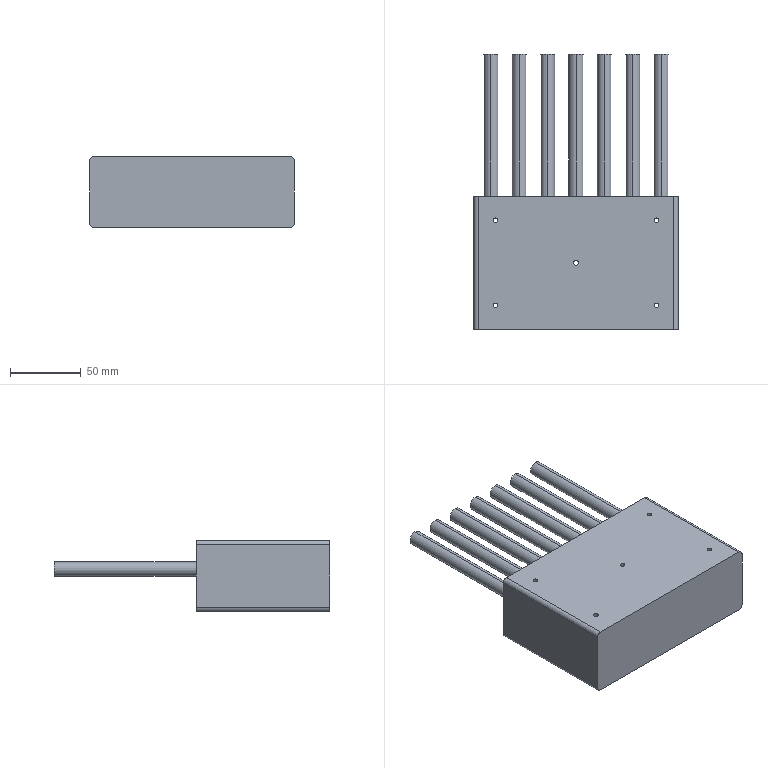Part | SolidWorks | features Extrusion 1, Fillet 1, HoleWzd 1, ICE 1 | 8 solids | 48 faces | box 144 x 194 x 50 mm | volume 728913 mm3 | cylinder 28 | plane 20 | commonest cylinder face diameters 10 x14 3.3 x10 6 x4
STEP:
#1=CARTESIAN_POINT('',(0.,147.,35.));
#2=VERTEX_POINT('',#1);
#3=CARTESIAN_POINT('',(0.,147.,25.));
#4=VERTEX_POINT('',#3);
#5=CARTESIAN_POINT('',(0.,147.,30.));
#6=DIRECTION('',(0.,1.,0.));
#7=DIRECTION('',(0.,0.,1.));
#8=AXIS2_PLACEMENT_3D('',#5,#6,#7);
#9=CIRCLE('',#8,5.);
#10=EDGE_CURVE('',#2,#4,#9,.T.);
#11=ORIENTED_EDGE('',*,*,#10,.F.);
#12=CARTESIAN_POINT('',(0.,47.,35.));
#13=VERTEX_POINT('',#12);
#14=CARTESIAN_POINT('',(0.,147.,35.));
#15=DIRECTION('',(0.,-1.,0.));
#16=VECTOR('',#15,1000.);
#17=LINE('',#14,#16);
#18=EDGE_CURVE('',#2,#13,#17,.T.);
#19=ORIENTED_EDGE('',*,*,#18,.T.);
#20=CARTESIAN_POINT('',(0.,47.,25.));
#21=VERTEX_POINT('',#20);
#22=CARTESIAN_POINT('',(0.,47.,30.));
#23=DIRECTION('',(0.,1.,0.));
#24=DIRECTION('',(0.,0.,1.));
#25=AXIS2_PLACEMENT_3D('',#22,#23,#24);
#26=CIRCLE('',#25,5.);
#27=EDGE_CURVE('',#13,#21,#26,.T.);
#28=ORIENTED_EDGE('',*,*,#27,.T.);
#29=CARTESIAN_POINT('',(0.,147.,25.));
#30=DIRECTION('',(0.,-1.,0.));
#31=VECTOR('',#30,1000.);
#32=LINE('',#29,#31);
#33=EDGE_CURVE('',#4,#21,#32,.T.);
#34=ORIENTED_EDGE('',*,*,#33,.F.);
#35=EDGE_LOOP('',(#11,#19,#28,#34));
#36=FACE_OUTER_BOUND('',#35,.T.);
#37=CARTESIAN_POINT('',(0.,147.,30.));
#38=DIRECTION('',(0.,-1.,0.));
#39=DIRECTION('',(0.,0.,-1.));
#40=AXIS2_PLACEMENT_3D('',#37,#38,#39);
#41=CYLINDRICAL_SURFACE('',#40,5.);
#42=ADVANCED_FACE('',(#36),#41,.T.);
#43=ORIENTED_EDGE('',*,*,#18,.F.);
#44=CARTESIAN_POINT('',(0.,147.,30.));
#45=DIRECTION('',(0.,1.,0.));
#46=DIRECTION('',(0.,0.,1.));
#47=AXIS2_PLACEMENT_3D('',#44,#45,#46);
#48=CIRCLE('',#47,5.);
#49=EDGE_CURVE('',#4,#2,#48,.T.);
#50=ORIENTED_EDGE('',*,*,#49,.F.);
#51=ORIENTED_EDGE('',*,*,#33,.T.);
#52=CARTESIAN_POINT('',(0.,47.,30.));
#53=DIRECTION('',(0.,1.,0.));
#54=DIRECTION('',(0.,0.,1.));
#55=AXIS2_PLACEMENT_3D('',#52,#53,#54);
#56=CIRCLE('',#55,5.);
#57=EDGE_CURVE('',#21,#13,#56,.T.);
#58=ORIENTED_EDGE('',*,*,#57,.T.);
#59=EDGE_LOOP('',(#43,#50,#51,#58));
#60=FACE_OUTER_BOUND('',#59,.T.);
#61=CARTESIAN_POINT('',(0.,147.,30.));
#62=DIRECTION('',(0.,-1.,0.));
#63=DIRECTION('',(0.,0.,-1.));
#64=AXIS2_PLACEMENT_3D('',#61,#62,#63);
#65=CYLINDRICAL_SURFACE('',#64,5.);
#66=ADVANCED_FACE('',(#60),#65,.T.);
#67=ORIENTED_EDGE('',*,*,#49,.T.);
#68=ORIENTED_EDGE('',*,*,#10,.T.);
#69=EDGE_LOOP('',(#67,#68));
#70=FACE_OUTER_BOUND('',#69,.T.);
#71=CARTESIAN_POINT('',(0.,147.,30.));
#72=DIRECTION('',(0.,1.,0.));
#73=DIRECTION('',(0.,0.,1.));
#74=AXIS2_PLACEMENT_3D('',#71,#72,#73);
#75=PLANE('',#74);
#76=ADVANCED_FACE('',(#70),#75,.T.);
#77=ORIENTED_EDGE('',*,*,#57,.F.);
#78=ORIENTED_EDGE('',*,*,#27,.F.);
#79=EDGE_LOOP('',(#77,#78));
#80=FACE_OUTER_BOUND('',#79,.T.);
#81=CARTESIAN_POINT('',(0.,47.,30.));
#82=DIRECTION('',(0.,1.,0.));
#83=DIRECTION('',(0.,0.,1.));
#84=AXIS2_PLACEMENT_3D('',#81,#82,#83);
#85=PLANE('',#84);
#86=ADVANCED_FACE('',(#80),#85,.F.);
#87=CLOSED_SHELL('',(#42,#66,#76,#86));
#88=MANIFOLD_SOLID_BREP('',#87);
#89=CARTESIAN_POINT('',(20.,147.,35.));
#90=VERTEX_POINT('',#89);
#91=CARTESIAN_POINT('',(20.,147.,25.));
#92=VERTEX_POINT('',#91);
#93=CARTESIAN_POINT('',(20.,147.,30.));
#94=DIRECTION('',(0.,1.,0.));
#95=DIRECTION('',(0.,0.,1.));
#96=AXIS2_PLACEMENT_3D('',#93,#94,#95);
#97=CIRCLE('',#96,5.);
#98=EDGE_CURVE('',#90,#92,#97,.T.);
#99=ORIENTED_EDGE('',*,*,#98,.F.);
#100=CARTESIAN_POINT('',(20.,47.,35.));
#101=VERTEX_POINT('',#100);
#102=CARTESIAN_POINT('',(20.,147.,35.));
#103=DIRECTION('',(0.,-1.,0.));
#104=VECTOR('',#103,1000.);
#105=LINE('',#102,#104);
#106=EDGE_CURVE('',#90,#101,#105,.T.);
#107=ORIENTED_EDGE('',*,*,#106,.T.);
#108=CARTESIAN_POINT('',(20.,47.,25.));
#109=VERTEX_POINT('',#108);
#110=CARTESIAN_POINT('',(20.,47.,30.));
#111=DIRECTION('',(0.,1.,0.));
#112=DIRECTION('',(0.,0.,1.));
#113=AXIS2_PLACEMENT_3D('',#110,#111,#112);
#114=CIRCLE('',#113,5.);
#115=EDGE_CURVE('',#101,#109,#114,.T.);
#116=ORIENTED_EDGE('',*,*,#115,.T.);
#117=CARTESIAN_POINT('',(20.,147.,25.));
#118=DIRECTION('',(0.,-1.,0.));
#119=VECTOR('',#118,1000.);
#120=LINE('',#117,#119);
#121=EDGE_CURVE('',#92,#109,#120,.T.);
#122=ORIENTED_EDGE('',*,*,#121,.F.);
#123=EDGE_LOOP('',(#99,#107,#116,#122));
#124=FACE_OUTER_BOUND('',#123,.T.);
#125=CARTESIAN_POINT('',(20.,147.,30.));
#126=DIRECTION('',(0.,-1.,0.));
#127=DIRECTION('',(0.,0.,-1.));
#128=AXIS2_PLACEMENT_3D('',#125,#126,#127);
#129=CYLINDRICAL_SURFACE('',#128,5.);
#130=ADVANCED_FACE('',(#124),#129,.T.);
#131=ORIENTED_EDGE('',*,*,#106,.F.);
#132=CARTESIAN_POINT('',(20.,147.,30.));
#133=DIRECTION('',(0.,1.,0.));
#134=DIRECTION('',(0.,0.,1.));
#135=AXIS2_PLACEMENT_3D('',#132,#133,#134);
#136=CIRCLE('',#135,5.);
#137=EDGE_CURVE('',#92,#90,#136,.T.);
#138=ORIENTED_EDGE('',*,*,#137,.F.);
#139=ORIENTED_EDGE('',*,*,#121,.T.);
#140=CARTESIAN_POINT('',(20.,47.,30.));
#141=DIRECTION('',(0.,1.,0.));
#142=DIRECTION('',(0.,0.,1.));
#143=AXIS2_PLACEMENT_3D('',#140,#141,#142);
#144=CIRCLE('',#143,5.);
#145=EDGE_CURVE('',#109,#101,#144,.T.);
#146=ORIENTED_EDGE('',*,*,#145,.T.);
#147=EDGE_LOOP('',(#131,#138,#139,#146));
#148=FACE_OUTER_BOUND('',#147,.T.);
#149=CARTESIAN_POINT('',(20.,147.,30.));
#150=DIRECTION('',(0.,-1.,0.));
#151=DIRECTION('',(0.,0.,-1.));
#152=AXIS2_PLACEMENT_3D('',#149,#150,#151);
#153=CYLINDRICAL_SURFACE('',#152,5.);
#154=ADVANCED_FACE('',(#148),#153,.T.);
#155=ORIENTED_EDGE('',*,*,#137,.T.);
#156=ORIENTED_EDGE('',*,*,#98,.T.);
#157=EDGE_LOOP('',(#155,#156));
#158=FACE_OUTER_BOUND('',#157,.T.);
#159=CARTESIAN_POINT('',(20.,147.,30.));
#160=DIRECTION('',(0.,1.,0.));
#161=DIRECTION('',(0.,0.,1.));
#162=AXIS2_PLACEMENT_3D('',#159,#160,#161);
#163=PLANE('',#162);
#164=ADVANCED_FACE('',(#158),#163,.T.);
#165=ORIENTED_EDGE('',*,*,#145,.F.);
#166=ORIENTED_EDGE('',*,*,#115,.F.);
#167=EDGE_LOOP('',(#165,#166));
#168=FACE_OUTER_BOUND('',#167,.T.);
#169=CARTESIAN_POINT('',(20.,47.,30.));
#170=DIRECTION('',(0.,1.,0.));
#171=DIRECTION('',(0.,0.,1.));
#172=AXIS2_PLACEMENT_3D('',#169,#170,#171);
#173=PLANE('',#172);
#174=ADVANCED_FACE('',(#168),#173,.F.);
#175=CLOSED_SHELL('',(#130,#154,#164,#174));
#176=MANIFOLD_SOLID_BREP('',#175);
#177=CARTESIAN_POINT('',(40.,147.,35.));
#178=VERTEX_POINT('',#177);
#179=CARTESIAN_POINT('',(40.,147.,25.));
#180=VERTEX_POINT('',#179);
#181=CARTESIAN_POINT('',(40.,147.,30.));
#182=DIRECTION('',(0.,1.,0.));
#183=DIRECTION('',(0.,0.,1.));
#184=AXIS2_PLACEMENT_3D('',#181,#182,#183);
#185=CIRCLE('',#184,5.);
#186=EDGE_CURVE('',#178,#180,#185,.T.);
#187=ORIENTED_EDGE('',*,*,#186,.F.);
#188=CARTESIAN_POINT('',(40.,47.,35.));
#189=VERTEX_POINT('',#188);
#190=CARTESIAN_POINT('',(40.,147.,35.));
#191=DIRECTION('',(0.,-1.,0.));
#192=VECTOR('',#191,1000.);
#193=LINE('',#190,#192);
#194=EDGE_CURVE('',#178,#189,#193,.T.);
#195=ORIENTED_EDGE('',*,*,#194,.T.);
#196=CARTESIAN_POINT('',(40.,47.,25.));
#197=VERTEX_POINT('',#196);
#198=CARTESIAN_POINT('',(40.,47.,30.));
#199=DIRECTION('',(0.,1.,0.));
#200=DIRECTION('',(0.,0.,1.));
#201=AXIS2_PLACEMENT_3D('',#198,#199,#200);
#202=CIRCLE('',#201,5.);
#203=EDGE_CURVE('',#189,#197,#202,.T.);
#204=ORIENTED_EDGE('',*,*,#203,.T.);
#205=CARTESIAN_POINT('',(40.,147.,25.));
#206=DIRECTION('',(0.,-1.,0.));
#207=VECTOR('',#206,1000.);
#208=LINE('',#205,#207);
#209=EDGE_CURVE('',#180,#197,#208,.T.);
#210=ORIENTED_EDGE('',*,*,#209,.F.);
#211=EDGE_LOOP('',(#187,#195,#204,#210));
#212=FACE_OUTER_BOUND('',#211,.T.);
#213=CARTESIAN_POINT('',(40.,147.,30.));
#214=DIRECTION('',(0.,-1.,0.));
#215=DIRECTION('',(0.,0.,-1.));
#216=AXIS2_PLACEMENT_3D('',#213,#214,#215);
#217=CYLINDRICAL_SURFACE('',#216,5.);
#218=ADVANCED_FACE('',(#212),#217,.T.);
#219=ORIENTED_EDGE('',*,*,#194,.F.);
#220=CARTESIAN_POINT('',(40.,147.,30.));
#221=DIRECTION('',(0.,1.,0.));
#222=DIRECTION('',(0.,0.,1.));
#223=AXIS2_PLACEMENT_3D('',#220,#221,#222);
#224=CIRCLE('',#223,5.);
#225=EDGE_CURVE('',#180,#178,#224,.T.);
#226=ORIENTED_EDGE('',*,*,#225,.F.);
#227=ORIENTED_EDGE('',*,*,#209,.T.);
#228=CARTESIAN_POINT('',(40.,47.,30.));
#229=DIRECTION('',(0.,1.,0.));
#230=DIRECTION('',(0.,0.,1.));
#231=AXIS2_PLACEMENT_3D('',#228,#229,#230);
#232=CIRCLE('',#231,5.);
#233=EDGE_CURVE('',#197,#189,#232,.T.);
#234=ORIENTED_EDGE('',*,*,#233,.T.);
#235=EDGE_LOOP('',(#219,#226,#227,#234));
#236=FACE_OUTER_BOUND('',#235,.T.);
#237=CARTESIAN_POINT('',(40.,147.,30.));
#238=DIRECTION('',(0.,-1.,0.));
#239=DIRECTION('',(0.,0.,-1.));
#240=AXIS2_PLACEMENT_3D('',#237,#238,#239);
#241=CYLINDRICAL_SURFACE('',#240,5.);
#242=ADVANCED_FACE('',(#236),#241,.T.);
#243=ORIENTED_EDGE('',*,*,#225,.T.);
#244=ORIENTED_EDGE('',*,*,#186,.T.);
#245=EDGE_LOOP('',(#243,#244));
#246=FACE_OUTER_BOUND('',#245,.T.);
#247=CARTESIAN_POINT('',(40.,147.,30.));
#248=DIRECTION('',(0.,1.,0.));
#249=DIRECTION('',(0.,0.,1.));
#250=AXIS2_PLACEMENT_3D('',#247,#248,#249);
#251=PLANE('',#250);
#252=ADVANCED_FACE('',(#246),#251,.T.);
#253=ORIENTED_EDGE('',*,*,#233,.F.);
#254=ORIENTED_EDGE('',*,*,#203,.F.);
#255=EDGE_LOOP('',(#253,#254));
#256=FACE_OUTER_BOUND('',#255,.T.);
#257=CARTESIAN_POINT('',(40.,47.,30.));
#258=DIRECTION('',(0.,1.,0.));
#259=DIRECTION('',(0.,0.,1.));
#260=AXIS2_PLACEMENT_3D('',#257,#258,#259);
#261=PLANE('',#260);
#262=ADVANCED_FACE('',(#256),#261,.F.);
#263=CLOSED_SHELL('',(#218,#242,#252,#262));
#264=MANIFOLD_SOLID_BREP('',#263);
#265=CARTESIAN_POINT('',(60.,147.,35.));
#266=VERTEX_POINT('',#265);
#267=CARTESIAN_POINT('',(60.,147.,25.));
#268=VERTEX_POINT('',#267);
#269=CARTESIAN_POINT('',(60.,147.,30.));
#270=DIRECTION('',(0.,1.,0.));
#271=DIRECTION('',(0.,0.,1.));
#272=AXIS2_PLACEMENT_3D('',#269,#270,#271);
#273=CIRCLE('',#272,5.);
#274=EDGE_CURVE('',#266,#268,#273,.T.);
#275=ORIENTED_EDGE('',*,*,#274,.F.);
#276=CARTESIAN_POINT('',(60.,47.,35.));
#277=VERTEX_POINT('',#276);
#278=CARTESIAN_POINT('',(60.,147.,35.));
#279=DIRECTION('',(0.,-1.,0.));
#280=VECTOR('',#279,1000.);
#281=LINE('',#278,#280);
#282=EDGE_CURVE('',#266,#277,#281,.T.);
#283=ORIENTED_EDGE('',*,*,#282,.T.);
#284=CARTESIAN_POINT('',(60.,47.,25.));
#285=VERTEX_POINT('',#284);
#286=CARTESIAN_POINT('',(60.,47.,30.));
#287=DIRECTION('',(0.,1.,0.));
#288=DIRECTION('',(0.,0.,1.));
#289=AXIS2_PLACEMENT_3D('',#286,#287,#288);
#290=CIRCLE('',#289,5.);
#291=EDGE_CURVE('',#277,#285,#290,.T.);
#292=ORIENTED_EDGE('',*,*,#291,.T.);
#293=CARTESIAN_POINT('',(60.,147.,25.));
#294=DIRECTION('',(0.,-1.,0.));
#295=VECTOR('',#294,1000.);
#296=LINE('',#293,#295);
#297=EDGE_CURVE('',#268,#285,#296,.T.);
#298=ORIENTED_EDGE('',*,*,#297,.F.);
#299=EDGE_LOOP('',(#275,#283,#292,#298));
#300=FACE_OUTER_BOUND('',#299,.T.);
#301=CARTESIAN_POINT('',(60.,147.,30.));
#302=DIRECTION('',(0.,-1.,0.));
#303=DIRECTION('',(0.,0.,-1.));
#304=AXIS2_PLACEMENT_3D('',#301,#302,#303);
#305=CYLINDRICAL_SURFACE('',#304,5.);
#306=ADVANCED_FACE('',(#300),#305,.T.);
#307=ORIENTED_EDGE('',*,*,#282,.F.);
#308=CARTESIAN_POINT('',(60.,147.,30.));
#309=DIRECTION('',(0.,1.,0.));
#310=DIRECTION('',(0.,0.,1.));
#311=AXIS2_PLACEMENT_3D('',#308,#309,#310);
#312=CIRCLE('',#311,5.);
#313=EDGE_CURVE('',#268,#266,#312,.T.);
#314=ORIENTED_EDGE('',*,*,#313,.F.);
#315=ORIENTED_EDGE('',*,*,#297,.T.);
#316=CARTESIAN_POINT('',(60.,47.,30.));
#317=DIRECTION('',(0.,1.,0.));
#318=DIRECTION('',(0.,0.,1.));
#319=AXIS2_PLACEMENT_3D('',#316,#317,#318);
#320=CIRCLE('',#319,5.);
#321=EDGE_CURVE('',#285,#277,#320,.T.);
#322=ORIENTED_EDGE('',*,*,#321,.T.);
#323=EDGE_LOOP('',(#307,#314,#315,#322));
#324=FACE_OUTER_BOUND('',#323,.T.);
#325=CARTESIAN_POINT('',(60.,147.,30.));
#326=DIRECTION('',(0.,-1.,0.));
#327=DIRECTION('',(0.,0.,-1.));
#328=AXIS2_PLACEMENT_3D('',#325,#326,#327);
#329=CYLINDRICAL_SURFACE('',#328,5.);
#330=ADVANCED_FACE('',(#324),#329,.T.);
#331=ORIENTED_EDGE('',*,*,#313,.T.);
#332=ORIENTED_EDGE('',*,*,#274,.T.);
#333=EDGE_LOOP('',(#331,#332));
#334=FACE_OUTER_BOUND('',#333,.T.);
#335=CARTESIAN_POINT('',(60.,147.,30.));
#336=DIRECTION('',(0.,1.,0.));
#337=DIRECTION('',(0.,0.,1.));
#338=AXIS2_PLACEMENT_3D('',#335,#336,#337);
#339=PLANE('',#338);
#340=ADVANCED_FACE('',(#334),#339,.T.);
#341=ORIENTED_EDGE('',*,*,#321,.F.);
#342=ORIENTED_EDGE('',*,*,#291,.F.);
#343=EDGE_LOOP('',(#341,#342));
#344=FACE_OUTER_BOUND('',#343,.T.);
#345=CARTESIAN_POINT('',(60.,47.,30.));
#346=DIRECTION('',(0.,1.,0.));
#347=DIRECTION('',(0.,0.,1.));
#348=AXIS2_PLACEMENT_3D('',#345,#346,#347);
#349=PLANE('',#348);
#350=ADVANCED_FACE('',(#344),#349,.F.);
#351=CLOSED_SHELL('',(#306,#330,#340,#350));
#352=MANIFOLD_SOLID_BREP('',#351);
#353=CARTESIAN_POINT('',(-60.,147.,35.));
#354=VERTEX_POINT('',#353);
#355=CARTESIAN_POINT('',(-60.,147.,25.));
#356=VERTEX_POINT('',#355);
#357=CARTESIAN_POINT('',(-60.,147.,30.));
#358=DIRECTION('',(0.,1.,0.));
#359=DIRECTION('',(0.,0.,-1.));
#360=AXIS2_PLACEMENT_3D('',#357,#358,#359);
#361=CIRCLE('',#360,5.);
#362=EDGE_CURVE('',#354,#356,#361,.T.);
#363=ORIENTED_EDGE('',*,*,#362,.F.);
#364=CARTESIAN_POINT('',(-60.,47.,35.));
#365=VERTEX_POINT('',#364);
#366=CARTESIAN_POINT('',(-60.,147.,35.));
#367=DIRECTION('',(0.,-1.,0.));
#368=VECTOR('',#367,1000.);
#369=LINE('',#366,#368);
#370=EDGE_CURVE('',#354,#365,#369,.T.);
#371=ORIENTED_EDGE('',*,*,#370,.T.);
#372=CARTESIAN_POINT('',(-60.,47.,25.));
#373=VERTEX_POINT('',#372);
#374=CARTESIAN_POINT('',(-60.,47.,30.));
#375=DIRECTION('',(0.,1.,0.));
#376=DIRECTION('',(0.,0.,-1.));
#377=AXIS2_PLACEMENT_3D('',#374,#375,#376);
#378=CIRCLE('',#377,5.);
#379=EDGE_CURVE('',#365,#373,#378,.T.);
#380=ORIENTED_EDGE('',*,*,#379,.T.);
#381=CARTESIAN_POINT('',(-60.,147.,25.));
#382=DIRECTION('',(0.,-1.,0.));
#383=VECTOR('',#382,1000.);
#384=LINE('',#381,#383);
#385=EDGE_CURVE('',#356,#373,#384,.T.);
#386=ORIENTED_EDGE('',*,*,#385,.F.);
#387=EDGE_LOOP('',(#363,#371,#380,#386));
#388=FACE_OUTER_BOUND('',#387,.T.);
#389=CARTESIAN_POINT('',(-60.,147.,30.));
#390=DIRECTION('',(0.,-1.,0.));
#391=DIRECTION('',(0.,0.,-1.));
#392=AXIS2_PLACEMENT_3D('',#389,#390,#391);
#393=CYLINDRICAL_SURFACE('',#392,5.);
#394=ADVANCED_FACE('',(#388),#393,.T.);
#395=ORIENTED_EDGE('',*,*,#370,.F.);
#396=CARTESIAN_POINT('',(-60.,147.,30.));
#397=DIRECTION('',(0.,1.,0.));
#398=DIRECTION('',(0.,0.,-1.));
#399=AXIS2_PLACEMENT_3D('',#396,#397,#398);
#400=CIRCLE('',#399,5.);
#401=EDGE_CURVE('',#356,#354,#400,.T.);
#402=ORIENTED_EDGE('',*,*,#401,.F.);
#403=ORIENTED_EDGE('',*,*,#385,.T.);
#404=CARTESIAN_POINT('',(-60.,47.,30.));
#405=DIRECTION('',(0.,1.,0.));
#406=DIRECTION('',(0.,0.,-1.));
#407=AXIS2_PLACEMENT_3D('',#404,#405,#406);
#408=CIRCLE('',#407,5.);
#409=EDGE_CURVE('',#373,#365,#408,.T.);
#410=ORIENTED_EDGE('',*,*,#409,.T.);
#411=EDGE_LOOP('',(#395,#402,#403,#410));
#412=FACE_OUTER_BOUND('',#411,.T.);
#413=CARTESIAN_POINT('',(-60.,147.,30.));
#414=DIRECTION('',(0.,-1.,0.));
#415=DIRECTION('',(0.,0.,-1.));
#416=AXIS2_PLACEMENT_3D('',#413,#414,#415);
#417=CYLINDRICAL_SURFACE('',#416,5.);
#418=ADVANCED_FACE('',(#412),#417,.T.);
#419=ORIENTED_EDGE('',*,*,#401,.T.);
#420=ORIENTED_EDGE('',*,*,#362,.T.);
#421=EDGE_LOOP('',(#419,#420));
#422=FACE_OUTER_BOUND('',#421,.T.);
#423=CARTESIAN_POINT('',(-60.,147.,30.));
#424=DIRECTION('',(0.,-1.,0.));
#425=DIRECTION('',(0.,0.,-1.));
#426=AXIS2_PLACEMENT_3D('',#423,#424,#425);
#427=PLANE('',#426);
#428=ADVANCED_FACE('',(#422),#427,.F.);
#429=ORIENTED_EDGE('',*,*,#409,.F.);
#430=ORIENTED_EDGE('',*,*,#379,.F.);
#431=EDGE_LOOP('',(#429,#430));
#432=FACE_OUTER_BOUND('',#431,.T.);
#433=CARTESIAN_POINT('',(-60.,47.,30.));
#434=DIRECTION('',(0.,-1.,0.));
#435=DIRECTION('',(0.,0.,-1.));
#436=AXIS2_PLACEMENT_3D('',#433,#434,#435);
#437=PLANE('',#436);
#438=ADVANCED_FACE('',(#432),#437,.T.);
#439=CLOSED_SHELL('',(#394,#418,#428,#438));
#440=MANIFOLD_SOLID_BREP('',#439);
#441=CARTESIAN_POINT('',(-40.,147.,35.));
#442=VERTEX_POINT('',#441);
#443=CARTESIAN_POINT('',(-40.,147.,25.));
#444=VERTEX_POINT('',#443);
#445=CARTESIAN_POINT('',(-40.,147.,30.));
#446=DIRECTION('',(0.,1.,0.));
#447=DIRECTION('',(0.,0.,-1.));
#448=AXIS2_PLACEMENT_3D('',#445,#446,#447);
#449=CIRCLE('',#448,5.);
#450=EDGE_CURVE('',#442,#444,#449,.T.);
#451=ORIENTED_EDGE('',*,*,#450,.F.);
#452=CARTESIAN_POINT('',(-40.,47.,35.));
#453=VERTEX_POINT('',#452);
#454=CARTESIAN_POINT('',(-40.,147.,35.));
#455=DIRECTION('',(0.,-1.,0.));
#456=VECTOR('',#455,1000.);
#457=LINE('',#454,#456);
#458=EDGE_CURVE('',#442,#453,#457,.T.);
#459=ORIENTED_EDGE('',*,*,#458,.T.);
#460=CARTESIAN_POINT('',(-40.,47.,25.));
#461=VERTEX_POINT('',#460);
#462=CARTESIAN_POINT('',(-40.,47.,30.));
#463=DIRECTION('',(0.,1.,0.));
#464=DIRECTION('',(0.,0.,-1.));
#465=AXIS2_PLACEMENT_3D('',#462,#463,#464);
#466=CIRCLE('',#465,5.);
#467=EDGE_CURVE('',#453,#461,#466,.T.);
#468=ORIENTED_EDGE('',*,*,#467,.T.);
#469=CARTESIAN_POINT('',(-40.,147.,25.));
#470=DIRECTION('',(0.,-1.,0.));
#471=VECTOR('',#470,1000.);
#472=LINE('',#469,#471);
#473=EDGE_CURVE('',#444,#461,#472,.T.);
#474=ORIENTED_EDGE('',*,*,#473,.F.);
#475=EDGE_LOOP('',(#451,#459,#468,#474));
#476=FACE_OUTER_BOUND('',#475,.T.);
#477=CARTESIAN_POINT('',(-40.,147.,30.));
#478=DIRECTION('',(0.,-1.,0.));
#479=DIRECTION('',(0.,0.,-1.));
#480=AXIS2_PLACEMENT_3D('',#477,#478,#479);
#481=CYLINDRICAL_SURFACE('',#480,5.);
#482=ADVANCED_FACE('',(#476),#481,.T.);
#483=ORIENTED_EDGE('',*,*,#458,.F.);
#484=CARTESIAN_POINT('',(-40.,147.,30.));
#485=DIRECTION('',(0.,1.,0.));
#486=DIRECTION('',(0.,0.,-1.));
#487=AXIS2_PLACEMENT_3D('',#484,#485,#486);
#488=CIRCLE('',#487,5.);
#489=EDGE_CURVE('',#444,#442,#488,.T.);
#490=ORIENTED_EDGE('',*,*,#489,.F.);
#491=ORIENTED_EDGE('',*,*,#473,.T.);
#492=CARTESIAN_POINT('',(-40.,47.,30.));
#493=DIRECTION('',(0.,1.,0.));
#494=DIRECTION('',(0.,0.,-1.));
#495=AXIS2_PLACEMENT_3D('',#492,#493,#494);
#496=CIRCLE('',#495,5.);
#497=EDGE_CURVE('',#461,#453,#496,.T.);
#498=ORIENTED_EDGE('',*,*,#497,.T.);
#499=EDGE_LOOP('',(#483,#490,#491,#498));
#500=FACE_OUTER_BOUND('',#499,.T.);
#501=CARTESIAN_POINT('',(-40.,147.,30.));
#502=DIRECTION('',(0.,-1.,0.));
#503=DIRECTION('',(0.,0.,-1.));
#504=AXIS2_PLACEMENT_3D('',#501,#502,#503);
#505=CYLINDRICAL_SURFACE('',#504,5.);
#506=ADVANCED_FACE('',(#500),#505,.T.);
#507=ORIENTED_EDGE('',*,*,#489,.T.);
#508=ORIENTED_EDGE('',*,*,#450,.T.);
#509=EDGE_LOOP('',(#507,#508));
#510=FACE_OUTER_BOUND('',#509,.T.);
#511=CARTESIAN_POINT('',(-40.,147.,30.));
#512=DIRECTION('',(0.,-1.,0.));
#513=DIRECTION('',(0.,0.,-1.));
#514=AXIS2_PLACEMENT_3D('',#511,#512,#513);
#515=PLANE('',#514);
#516=ADVANCED_FACE('',(#510),#515,.F.);
#517=ORIENTED_EDGE('',*,*,#497,.F.);
#518=ORIENTED_EDGE('',*,*,#467,.F.);
#519=EDGE_LOOP('',(#517,#518));
#520=FACE_OUTER_BOUND('',#519,.T.);
#521=CARTESIAN_POINT('',(-40.,47.,30.));
#522=DIRECTION('',(0.,-1.,0.));
#523=DIRECTION('',(0.,0.,-1.));
#524=AXIS2_PLACEMENT_3D('',#521,#522,#523);
#525=PLANE('',#524);
#526=ADVANCED_FACE('',(#520),#525,.T.);
#527=CLOSED_SHELL('',(#482,#506,#516,#526));
#528=MANIFOLD_SOLID_BREP('',#527);
#529=CARTESIAN_POINT('',(-20.,147.,35.));
#530=VERTEX_POINT('',#529);
#531=CARTESIAN_POINT('',(-20.,147.,25.));
#532=VERTEX_POINT('',#531);
#533=CARTESIAN_POINT('',(-20.,147.,30.));
#534=DIRECTION('',(0.,1.,0.));
#535=DIRECTION('',(0.,0.,-1.));
#536=AXIS2_PLACEMENT_3D('',#533,#534,#535);
#537=CIRCLE('',#536,5.);
#538=EDGE_CURVE('',#530,#532,#537,.T.);
#539=ORIENTED_EDGE('',*,*,#538,.F.);
#540=CARTESIAN_POINT('',(-20.,47.,35.));
#541=VERTEX_POINT('',#540);
#542=CARTESIAN_POINT('',(-20.,147.,35.));
#543=DIRECTION('',(0.,-1.,0.));
#544=VECTOR('',#543,1000.);
#545=LINE('',#542,#544);
#546=EDGE_CURVE('',#530,#541,#545,.T.);
#547=ORIENTED_EDGE('',*,*,#546,.T.);
#548=CARTESIAN_POINT('',(-20.,47.,25.));
#549=VERTEX_POINT('',#548);
#550=CARTESIAN_POINT('',(-20.,47.,30.));
#551=DIRECTION('',(0.,1.,0.));
#552=DIRECTION('',(0.,0.,-1.));
#553=AXIS2_PLACEMENT_3D('',#550,#551,#552);
#554=CIRCLE('',#553,5.);
#555=EDGE_CURVE('',#541,#549,#554,.T.);
#556=ORIENTED_EDGE('',*,*,#555,.T.);
#557=CARTESIAN_POINT('',(-20.,147.,25.));
#558=DIRECTION('',(0.,-1.,0.));
#559=VECTOR('',#558,1000.);
#560=LINE('',#557,#559);
#561=EDGE_CURVE('',#532,#549,#560,.T.);
#562=ORIENTED_EDGE('',*,*,#561,.F.);
#563=EDGE_LOOP('',(#539,#547,#556,#562));
#564=FACE_OUTER_BOUND('',#563,.T.);
#565=CARTESIAN_POINT('',(-20.,147.,30.));
#566=DIRECTION('',(0.,-1.,0.));
#567=DIRECTION('',(0.,0.,-1.));
#568=AXIS2_PLACEMENT_3D('',#565,#566,#567);
#569=CYLINDRICAL_SURFACE('',#568,5.);
#570=ADVANCED_FACE('',(#564),#569,.T.);
#571=ORIENTED_EDGE('',*,*,#546,.F.);
#572=CARTESIAN_POINT('',(-20.,147.,30.));
#573=DIRECTION('',(0.,1.,0.));
#574=DIRECTION('',(0.,0.,-1.));
#575=AXIS2_PLACEMENT_3D('',#572,#573,#574);
#576=CIRCLE('',#575,5.);
#577=EDGE_CURVE('',#532,#530,#576,.T.);
#578=ORIENTED_EDGE('',*,*,#577,.F.);
#579=ORIENTED_EDGE('',*,*,#561,.T.);
#580=CARTESIAN_POINT('',(-20.,47.,30.));
#581=DIRECTION('',(0.,1.,0.));
#582=DIRECTION('',(0.,0.,-1.));
#583=AXIS2_PLACEMENT_3D('',#580,#581,#582);
#584=CIRCLE('',#583,5.);
#585=EDGE_CURVE('',#549,#541,#584,.T.);
#586=ORIENTED_EDGE('',*,*,#585,.T.);
#587=EDGE_LOOP('',(#571,#578,#579,#586));
#588=FACE_OUTER_BOUND('',#587,.T.);
#589=CARTESIAN_POINT('',(-20.,147.,30.));
#590=DIRECTION('',(0.,-1.,0.));
#591=DIRECTION('',(0.,0.,-1.));
#592=AXIS2_PLACEMENT_3D('',#589,#590,#591);
#593=CYLINDRICAL_SURFACE('',#592,5.);
#594=ADVANCED_FACE('',(#588),#593,.T.);
#595=ORIENTED_EDGE('',*,*,#577,.T.);
#596=ORIENTED_EDGE('',*,*,#538,.T.);
#597=EDGE_LOOP('',(#595,#596));
#598=FACE_OUTER_BOUND('',#597,.T.);
#599=CARTESIAN_POINT('',(-20.,147.,30.));
#600=DIRECTION('',(0.,-1.,0.));
#601=DIRECTION('',(0.,0.,-1.));
#602=AXIS2_PLACEMENT_3D('',#599,#600,#601);
#603=PLANE('',#602);
#604=ADVANCED_FACE('',(#598),#603,.F.);
#605=ORIENTED_EDGE('',*,*,#585,.F.);
#606=ORIENTED_EDGE('',*,*,#555,.F.);
#607=EDGE_LOOP('',(#605,#606));
#608=FACE_OUTER_BOUND('',#607,.T.);
#609=CARTESIAN_POINT('',(-20.,47.,30.));
#610=DIRECTION('',(0.,-1.,0.));
#611=DIRECTION('',(0.,0.,-1.));
#612=AXIS2_PLACEMENT_3D('',#609,#610,#611);
#613=PLANE('',#612);
#614=ADVANCED_FACE('',(#608),#613,.T.);
#615=CLOSED_SHELL('',(#570,#594,#604,#614));
#616=MANIFOLD_SOLID_BREP('',#615);
#617=CARTESIAN_POINT('',(-58.4,30.,0.));
#618=VERTEX_POINT('',#617);
#619=CARTESIAN_POINT('',(-55.1,30.,0.));
#620=VERTEX_POINT('',#619);
#621=CARTESIAN_POINT('',(-56.75,30.,0.));
#622=DIRECTION('',(0.,0.,1.));
#623=DIRECTION('',(1.,0.,0.));
#624=AXIS2_PLACEMENT_3D('',#621,#622,#623);
#625=CIRCLE('',#624,1.65);
#626=EDGE_CURVE('',#618,#620,#625,.T.);
#627=ORIENTED_EDGE('',*,*,#626,.F.);
#628=CARTESIAN_POINT('',(-58.4,30.,50.));
#629=VERTEX_POINT('',#628);
#630=CARTESIAN_POINT('',(-58.4,30.,50.));
#631=DIRECTION('',(0.,0.,1.));
#632=VECTOR('',#631,1000.);
#633=LINE('',#630,#632);
#634=EDGE_CURVE('',#618,#629,#633,.T.);
#635=ORIENTED_EDGE('',*,*,#634,.T.);
#636=CARTESIAN_POINT('',(-55.1,30.,50.));
#637=VERTEX_POINT('',#636);
#638=CARTESIAN_POINT('',(-56.75,30.,50.));
#639=DIRECTION('',(0.,0.,1.));
#640=DIRECTION('',(1.,0.,0.));
#641=AXIS2_PLACEMENT_3D('',#638,#639,#640);
#642=CIRCLE('',#641,1.65);
#643=EDGE_CURVE('',#629,#637,#642,.T.);
#644=ORIENTED_EDGE('',*,*,#643,.T.);
#645=CARTESIAN_POINT('',(-55.1,30.,50.));
#646=DIRECTION('',(0.,0.,1.));
#647=VECTOR('',#646,1000.);
#648=LINE('',#645,#647);
#649=EDGE_CURVE('',#620,#637,#648,.T.);
#650=ORIENTED_EDGE('',*,*,#649,.F.);
#651=EDGE_LOOP('',(#627,#635,#644,#650));
#652=FACE_OUTER_BOUND('',#651,.T.);
#653=CARTESIAN_POINT('',(-56.75,30.,50.));
#654=DIRECTION('',(0.,0.,1.));
#655=DIRECTION('',(1.,0.,0.));
#656=AXIS2_PLACEMENT_3D('',#653,#654,#655);
#657=CYLINDRICAL_SURFACE('',#656,1.65);
#658=ADVANCED_FACE('',(#652),#657,.F.);
#659=CARTESIAN_POINT('',(-1.65,0.,0.));
#660=VERTEX_POINT('',#659);
#661=CARTESIAN_POINT('',(1.65,0.,0.));
#662=VERTEX_POINT('',#661);
#663=CARTESIAN_POINT('',(0.,0.,0.));
#664=DIRECTION('',(0.,0.,1.));
#665=DIRECTION('',(1.,0.,0.));
#666=AXIS2_PLACEMENT_3D('',#663,#664,#665);
#667=CIRCLE('',#666,1.65);
#668=EDGE_CURVE('',#660,#662,#667,.T.);
#669=ORIENTED_EDGE('',*,*,#668,.F.);
#670=CARTESIAN_POINT('',(-1.65,0.,50.));
#671=VERTEX_POINT('',#670);
#672=CARTESIAN_POINT('',(-1.65,0.,50.));
#673=DIRECTION('',(0.,0.,1.));
#674=VECTOR('',#673,1000.);
#675=LINE('',#672,#674);
#676=EDGE_CURVE('',#660,#671,#675,.T.);
#677=ORIENTED_EDGE('',*,*,#676,.T.);
#678=CARTESIAN_POINT('',(1.65,0.,50.));
#679=VERTEX_POINT('',#678);
#680=CARTESIAN_POINT('',(0.,0.,50.));
#681=DIRECTION('',(0.,0.,1.));
#682=DIRECTION('',(1.,0.,0.));
#683=AXIS2_PLACEMENT_3D('',#680,#681,#682);
#684=CIRCLE('',#683,1.65);
#685=EDGE_CURVE('',#671,#679,#684,.T.);
#686=ORIENTED_EDGE('',*,*,#685,.T.);
#687=CARTESIAN_POINT('',(1.65,0.,50.));
#688=DIRECTION('',(0.,0.,1.));
#689=VECTOR('',#688,1000.);
#690=LINE('',#687,#689);
#691=EDGE_CURVE('',#662,#679,#690,.T.);
#692=ORIENTED_EDGE('',*,*,#691,.F.);
#693=EDGE_LOOP('',(#669,#677,#686,#692));
#694=FACE_OUTER_BOUND('',#693,.T.);
#695=CARTESIAN_POINT('',(0.,0.,50.));
#696=DIRECTION('',(0.,0.,1.));
#697=DIRECTION('',(1.,0.,0.));
#698=AXIS2_PLACEMENT_3D('',#695,#696,#697);
#699=CYLINDRICAL_SURFACE('',#698,1.65);
#700=ADVANCED_FACE('',(#694),#699,.F.);
#701=CARTESIAN_POINT('',(55.1,30.,0.));
#702=VERTEX_POINT('',#701);
#703=CARTESIAN_POINT('',(58.4,30.,0.));
#704=VERTEX_POINT('',#703);
#705=CARTESIAN_POINT('',(56.75,30.,0.));
#706=DIRECTION('',(0.,0.,1.));
#707=DIRECTION('',(1.,0.,0.));
#708=AXIS2_PLACEMENT_3D('',#705,#706,#707);
#709=CIRCLE('',#708,1.65);
#710=EDGE_CURVE('',#702,#704,#709,.T.);
#711=ORIENTED_EDGE('',*,*,#710,.F.);
#712=CARTESIAN_POINT('',(55.1,30.,50.));
#713=VERTEX_POINT('',#712);
#714=CARTESIAN_POINT('',(55.1,30.,50.));
#715=DIRECTION('',(0.,0.,1.));
#716=VECTOR('',#715,1000.);
#717=LINE('',#714,#716);
#718=EDGE_CURVE('',#702,#713,#717,.T.);
#719=ORIENTED_EDGE('',*,*,#718,.T.);
#720=CARTESIAN_POINT('',(58.4,30.,50.));
#721=VERTEX_POINT('',#720);
#722=CARTESIAN_POINT('',(56.75,30.,50.));
#723=DIRECTION('',(0.,0.,1.));
#724=DIRECTION('',(1.,0.,0.));
#725=AXIS2_PLACEMENT_3D('',#722,#723,#724);
#726=CIRCLE('',#725,1.65);
#727=EDGE_CURVE('',#713,#721,#726,.T.);
#728=ORIENTED_EDGE('',*,*,#727,.T.);
#729=CARTESIAN_POINT('',(58.4,30.,50.));
#730=DIRECTION('',(0.,0.,1.));
#731=VECTOR('',#730,1000.);
#732=LINE('',#729,#731);
#733=EDGE_CURVE('',#704,#721,#732,.T.);
#734=ORIENTED_EDGE('',*,*,#733,.F.);
#735=EDGE_LOOP('',(#711,#719,#728,#734));
#736=FACE_OUTER_BOUND('',#735,.T.);
#737=CARTESIAN_POINT('',(56.75,30.,50.));
#738=DIRECTION('',(0.,0.,1.));
#739=DIRECTION('',(1.,0.,0.));
#740=AXIS2_PLACEMENT_3D('',#737,#738,#739);
#741=CYLINDRICAL_SURFACE('',#740,1.65);
#742=ADVANCED_FACE('',(#736),#741,.F.);
#743=CARTESIAN_POINT('',(-58.4,-30.,0.));
#744=VERTEX_POINT('',#743);
#745=CARTESIAN_POINT('',(-55.1,-30.,0.));
#746=VERTEX_POINT('',#745);
#747=CARTESIAN_POINT('',(-56.75,-30.,0.));
#748=DIRECTION('',(0.,0.,1.));
#749=DIRECTION('',(1.,0.,0.));
#750=AXIS2_PLACEMENT_3D('',#747,#748,#749);
#751=CIRCLE('',#750,1.65);
#752=EDGE_CURVE('',#744,#746,#751,.T.);
#753=ORIENTED_EDGE('',*,*,#752,.F.);
#754=CARTESIAN_POINT('',(-58.4,-30.,50.));
#755=VERTEX_POINT('',#754);
#756=CARTESIAN_POINT('',(-58.4,-30.,50.));
#757=DIRECTION('',(0.,0.,1.));
#758=VECTOR('',#757,1000.);
#759=LINE('',#756,#758);
#760=EDGE_CURVE('',#744,#755,#759,.T.);
#761=ORIENTED_EDGE('',*,*,#760,.T.);
#762=CARTESIAN_POINT('',(-55.1,-30.,50.));
#763=VERTEX_POINT('',#762);
#764=CARTESIAN_POINT('',(-56.75,-30.,50.));
#765=DIRECTION('',(0.,0.,1.));
#766=DIRECTION('',(1.,0.,0.));
#767=AXIS2_PLACEMENT_3D('',#764,#765,#766);
#768=CIRCLE('',#767,1.65);
#769=EDGE_CURVE('',#755,#763,#768,.T.);
#770=ORIENTED_EDGE('',*,*,#769,.T.);
#771=CARTESIAN_POINT('',(-55.1,-30.,50.));
#772=DIRECTION('',(0.,0.,1.));
#773=VECTOR('',#772,1000.);
#774=LINE('',#771,#773);
#775=EDGE_CURVE('',#746,#763,#774,.T.);
#776=ORIENTED_EDGE('',*,*,#775,.F.);
#777=EDGE_LOOP('',(#753,#761,#770,#776));
#778=FACE_OUTER_BOUND('',#777,.T.);
#779=CARTESIAN_POINT('',(-56.75,-30.,50.));
#780=DIRECTION('',(0.,0.,1.));
#781=DIRECTION('',(1.,0.,0.));
#782=AXIS2_PLACEMENT_3D('',#779,#780,#781);
#783=CYLINDRICAL_SURFACE('',#782,1.65);
#784=ADVANCED_FACE('',(#778),#783,.F.);
#785=CARTESIAN_POINT('',(55.1,-30.,0.));
#786=VERTEX_POINT('',#785);
#787=CARTESIAN_POINT('',(58.4,-30.,0.));
#788=VERTEX_POINT('',#787);
#789=CARTESIAN_POINT('',(56.75,-30.,0.));
#790=DIRECTION('',(0.,0.,1.));
#791=DIRECTION('',(1.,0.,0.));
#792=AXIS2_PLACEMENT_3D('',#789,#790,#791);
#793=CIRCLE('',#792,1.65);
#794=EDGE_CURVE('',#786,#788,#793,.T.);
#795=ORIENTED_EDGE('',*,*,#794,.F.);
#796=CARTESIAN_POINT('',(55.1,-30.,50.));
#797=VERTEX_POINT('',#796);
#798=CARTESIAN_POINT('',(55.1,-30.,50.));
#799=DIRECTION('',(0.,0.,1.));
#800=VECTOR('',#799,1000.);
#801=LINE('',#798,#800);
#802=EDGE_CURVE('',#786,#797,#801,.T.);
#803=ORIENTED_EDGE('',*,*,#802,.T.);
#804=CARTESIAN_POINT('',(58.4,-30.,50.));
#805=VERTEX_POINT('',#804);
#806=CARTESIAN_POINT('',(56.75,-30.,50.));
#807=DIRECTION('',(0.,0.,1.));
#808=DIRECTION('',(1.,0.,0.));
#809=AXIS2_PLACEMENT_3D('',#806,#807,#808);
#810=CIRCLE('',#809,1.65);
#811=EDGE_CURVE('',#797,#805,#810,.T.);
#812=ORIENTED_EDGE('',*,*,#811,.T.);
#813=CARTESIAN_POINT('',(58.4,-30.,50.));
#814=DIRECTION('',(0.,0.,1.));
#815=VECTOR('',#814,1000.);
#816=LINE('',#813,#815);
#817=EDGE_CURVE('',#788,#805,#816,.T.);
#818=ORIENTED_EDGE('',*,*,#817,.F.);
#819=EDGE_LOOP('',(#795,#803,#812,#818));
#820=FACE_OUTER_BOUND('',#819,.T.);
#821=CARTESIAN_POINT('',(56.75,-30.,50.));
#822=DIRECTION('',(0.,0.,1.));
#823=DIRECTION('',(1.,0.,0.));
#824=AXIS2_PLACEMENT_3D('',#821,#822,#823);
#825=CYLINDRICAL_SURFACE('',#824,1.65);
#826=ADVANCED_FACE('',(#820),#825,.F.);
#827=CARTESIAN_POINT('',(72.,-47.,47.));
#828=VERTEX_POINT('',#827);
#829=CARTESIAN_POINT('',(72.,-47.,3.));
#830=VERTEX_POINT('',#829);
#831=CARTESIAN_POINT('',(72.,-47.,50.));
#832=DIRECTION('',(0.,0.,-1.));
#833=VECTOR('',#832,1000.);
#834=LINE('',#831,#833);
#835=EDGE_CURVE('',#828,#830,#834,.T.);
#836=ORIENTED_EDGE('',*,*,#835,.T.);
#837=CARTESIAN_POINT('',(72.,47.,3.));
#838=VERTEX_POINT('',#837);
#839=CARTESIAN_POINT('',(72.,47.,3.));
#840=DIRECTION('',(0.,1.,0.));
#841=VECTOR('',#840,1000.);
#842=LINE('',#839,#841);
#843=EDGE_CURVE('',#830,#838,#842,.T.);
#844=ORIENTED_EDGE('',*,*,#843,.T.);
#845=CARTESIAN_POINT('',(72.,47.,47.));
#846=VERTEX_POINT('',#845);
#847=CARTESIAN_POINT('',(72.,47.,50.));
#848=DIRECTION('',(0.,0.,-1.));
#849=VECTOR('',#848,1000.);
#850=LINE('',#847,#849);
#851=EDGE_CURVE('',#846,#838,#850,.T.);
#852=ORIENTED_EDGE('',*,*,#851,.F.);
#853=CARTESIAN_POINT('',(72.,-47.,47.));
#854=DIRECTION('',(0.,-1.,0.));
#855=VECTOR('',#854,1000.);
#856=LINE('',#853,#855);
#857=EDGE_CURVE('',#846,#828,#856,.T.);
#858=ORIENTED_EDGE('',*,*,#857,.T.);
#859=EDGE_LOOP('',(#836,#844,#852,#858));
#860=FACE_OUTER_BOUND('',#859,.T.);
#861=CARTESIAN_POINT('',(72.,-47.,50.));
#862=DIRECTION('',(-1.,0.,0.));
#863=DIRECTION('',(0.,0.,1.));
#864=AXIS2_PLACEMENT_3D('',#861,#862,#863);
#865=PLANE('',#864);
#866=ADVANCED_FACE('',(#860),#865,.F.);
#867=ORIENTED_EDGE('',*,*,#851,.T.);
#868=CARTESIAN_POINT('',(69.,47.,0.));
#869=VERTEX_POINT('',#868);
#870=CARTESIAN_POINT('',(69.,47.,3.));
#871=DIRECTION('',(0.,1.,0.));
#872=DIRECTION('',(0.,0.,-1.));
#873=AXIS2_PLACEMENT_3D('',#870,#871,#872);
#874=CIRCLE('',#873,3.);
#875=EDGE_CURVE('',#838,#869,#874,.T.);
#876=ORIENTED_EDGE('',*,*,#875,.T.);
#877=CARTESIAN_POINT('',(-69.,47.,0.));
#878=VERTEX_POINT('',#877);
#879=CARTESIAN_POINT('',(-72.,47.,0.));
#880=DIRECTION('',(-1.,0.,0.));
#881=VECTOR('',#880,1000.);
#882=LINE('',#879,#881);
#883=EDGE_CURVE('',#869,#878,#882,.T.);
#884=ORIENTED_EDGE('',*,*,#883,.T.);
#885=CARTESIAN_POINT('',(-72.,47.,3.));
#886=VERTEX_POINT('',#885);
#887=CARTESIAN_POINT('',(-69.,47.,3.));
#888=DIRECTION('',(0.,1.,0.));
#889=DIRECTION('',(0.,0.,-1.));
#890=AXIS2_PLACEMENT_3D('',#887,#888,#889);
#891=CIRCLE('',#890,3.);
#892=EDGE_CURVE('',#878,#886,#891,.T.);
#893=ORIENTED_EDGE('',*,*,#892,.T.);
#894=CARTESIAN_POINT('',(-72.,47.,47.));
#895=VERTEX_POINT('',#894);
#896=CARTESIAN_POINT('',(-72.,47.,50.));
#897=DIRECTION('',(0.,0.,-1.));
#898=VECTOR('',#897,1000.);
#899=LINE('',#896,#898);
#900=EDGE_CURVE('',#895,#886,#899,.T.);
#901=ORIENTED_EDGE('',*,*,#900,.F.);
#902=CARTESIAN_POINT('',(-69.,47.,50.));
#903=VERTEX_POINT('',#902);
#904=CARTESIAN_POINT('',(-69.,47.,47.));
#905=DIRECTION('',(0.,1.,0.));
#906=DIRECTION('',(0.,0.,-1.));
#907=AXIS2_PLACEMENT_3D('',#904,#905,#906);
#908=CIRCLE('',#907,3.);
#909=EDGE_CURVE('',#895,#903,#908,.T.);
#910=ORIENTED_EDGE('',*,*,#909,.T.);
#911=CARTESIAN_POINT('',(69.,47.,50.));
#912=VERTEX_POINT('',#911);
#913=CARTESIAN_POINT('',(-72.,47.,50.));
#914=DIRECTION('',(-1.,0.,0.));
#915=VECTOR('',#914,1000.);
#916=LINE('',#913,#915);
#917=EDGE_CURVE('',#912,#903,#916,.T.);
#918=ORIENTED_EDGE('',*,*,#917,.F.);
#919=CARTESIAN_POINT('',(69.,47.,47.));
#920=DIRECTION('',(0.,1.,0.));
#921=DIRECTION('',(0.,0.,-1.));
#922=AXIS2_PLACEMENT_3D('',#919,#920,#921);
#923=CIRCLE('',#922,3.);
#924=EDGE_CURVE('',#912,#846,#923,.T.);
#925=ORIENTED_EDGE('',*,*,#924,.T.);
#926=EDGE_LOOP('',(#867,#876,#884,#893,#901,#910,#918,#925));
#927=FACE_OUTER_BOUND('',#926,.T.);
#928=CARTESIAN_POINT('',(-72.,47.,50.));
#929=DIRECTION('',(0.,-1.,0.));
#930=DIRECTION('',(0.,0.,-1.));
#931=AXIS2_PLACEMENT_3D('',#928,#929,#930);
#932=PLANE('',#931);
#933=ADVANCED_FACE('',(#927),#932,.F.);
#934=ORIENTED_EDGE('',*,*,#900,.T.);
#935=CARTESIAN_POINT('',(-72.,-47.,3.));
#936=VERTEX_POINT('',#935);
#937=CARTESIAN_POINT('',(-72.,-47.,3.));
#938=DIRECTION('',(0.,-1.,0.));
#939=VECTOR('',#938,1000.);
#940=LINE('',#937,#939);
#941=EDGE_CURVE('',#886,#936,#940,.T.);
#942=ORIENTED_EDGE('',*,*,#941,.T.);
#943=CARTESIAN_POINT('',(-72.,-47.,47.));
#944=VERTEX_POINT('',#943);
#945=CARTESIAN_POINT('',(-72.,-47.,50.));
#946=DIRECTION('',(0.,0.,-1.));
#947=VECTOR('',#946,1000.);
#948=LINE('',#945,#947);
#949=EDGE_CURVE('',#944,#936,#948,.T.);
#950=ORIENTED_EDGE('',*,*,#949,.F.);
#951=CARTESIAN_POINT('',(-72.,-47.,47.));
#952=DIRECTION('',(0.,1.,0.));
#953=VECTOR('',#952,1000.);
#954=LINE('',#951,#953);
#955=EDGE_CURVE('',#944,#895,#954,.T.);
#956=ORIENTED_EDGE('',*,*,#955,.T.);
#957=EDGE_LOOP('',(#934,#942,#950,#956));
#958=FACE_OUTER_BOUND('',#957,.T.);
#959=CARTESIAN_POINT('',(-72.,-47.,50.));
#960=DIRECTION('',(1.,0.,0.));
#961=DIRECTION('',(0.,0.,-1.));
#962=AXIS2_PLACEMENT_3D('',#959,#960,#961);
#963=PLANE('',#962);
#964=ADVANCED_FACE('',(#958),#963,.F.);
#965=CARTESIAN_POINT('',(-69.,-47.,0.));
#966=VERTEX_POINT('',#965);
#967=CARTESIAN_POINT('',(69.,-47.,0.));
#968=VERTEX_POINT('',#967);
#969=CARTESIAN_POINT('',(-72.,-47.,0.));
#970=DIRECTION('',(1.,0.,0.));
#971=VECTOR('',#970,1000.);
#972=LINE('',#969,#971);
#973=EDGE_CURVE('',#966,#968,#972,.T.);
#974=ORIENTED_EDGE('',*,*,#973,.T.);
#975=CARTESIAN_POINT('',(69.,-47.,3.));
#976=DIRECTION('',(0.,-1.,0.));
#977=DIRECTION('',(0.,0.,1.));
#978=AXIS2_PLACEMENT_3D('',#975,#976,#977);
#979=CIRCLE('',#978,3.);
#980=EDGE_CURVE('',#968,#830,#979,.T.);
#981=ORIENTED_EDGE('',*,*,#980,.T.);
#982=ORIENTED_EDGE('',*,*,#835,.F.);
#983=CARTESIAN_POINT('',(69.,-47.,50.));
#984=VERTEX_POINT('',#983);
#985=CARTESIAN_POINT('',(69.,-47.,47.));
#986=DIRECTION('',(0.,-1.,0.));
#987=DIRECTION('',(0.,0.,1.));
#988=AXIS2_PLACEMENT_3D('',#985,#986,#987);
#989=CIRCLE('',#988,3.);
#990=EDGE_CURVE('',#828,#984,#989,.T.);
#991=ORIENTED_EDGE('',*,*,#990,.T.);
#992=CARTESIAN_POINT('',(-69.,-47.,50.));
#993=VERTEX_POINT('',#992);
#994=CARTESIAN_POINT('',(-72.,-47.,50.));
#995=DIRECTION('',(1.,0.,0.));
#996=VECTOR('',#995,1000.);
#997=LINE('',#994,#996);
#998=EDGE_CURVE('',#993,#984,#997,.T.);
#999=ORIENTED_EDGE('',*,*,#998,.F.);
#1000=CARTESIAN_POINT('',(-69.,-47.,47.));
#1001=DIRECTION('',(0.,-1.,0.));
#1002=DIRECTION('',(0.,0.,1.));
#1003=AXIS2_PLACEMENT_3D('',#1000,#1001,#1002);
#1004=CIRCLE('',#1003,3.);
#1005=EDGE_CURVE('',#993,#944,#1004,.T.);
#1006=ORIENTED_EDGE('',*,*,#1005,.T.);
#1007=ORIENTED_EDGE('',*,*,#949,.T.);
#1008=CARTESIAN_POINT('',(-69.,-47.,3.));
#1009=DIRECTION('',(0.,-1.,0.));
#1010=DIRECTION('',(0.,0.,1.));
#1011=AXIS2_PLACEMENT_3D('',#1008,#1009,#1010);
#1012=CIRCLE('',#1011,3.);
#1013=EDGE_CURVE('',#936,#966,#1012,.T.);
#1014=ORIENTED_EDGE('',*,*,#1013,.T.);
#1015=EDGE_LOOP('',(#974,#981,#982,#991,#999,#1006,#1007,#1014));
#1016=FACE_OUTER_BOUND('',#1015,.T.);
#1017=CARTESIAN_POINT('',(-72.,-47.,50.));
#1018=DIRECTION('',(0.,1.,0.));
#1019=DIRECTION('',(0.,0.,1.));
#1020=AXIS2_PLACEMENT_3D('',#1017,#1018,#1019);
#1021=PLANE('',#1020);
#1022=ADVANCED_FACE('',(#1016),#1021,.F.);
#1023=CARTESIAN_POINT('',(-56.75,30.,50.));
#1024=DIRECTION('',(0.,0.,1.));
#1025=DIRECTION('',(1.,0.,0.));
#1026=AXIS2_PLACEMENT_3D('',#1023,#1024,#1025);
#1027=CIRCLE('',#1026,1.65);
#1028=EDGE_CURVE('',#637,#629,#1027,.T.);
#1029=ORIENTED_EDGE('',*,*,#1028,.F.);
#1030=ORIENTED_EDGE('',*,*,#643,.F.);
#1031=EDGE_LOOP('',(#1029,#1030));
#1032=FACE_BOUND('',#1031,.T.);
#1033=CARTESIAN_POINT('',(0.,0.,50.));
#1034=DIRECTION('',(0.,0.,1.));
#1035=DIRECTION('',(1.,0.,0.));
#1036=AXIS2_PLACEMENT_3D('',#1033,#1034,#1035);
#1037=CIRCLE('',#1036,1.65);
#1038=EDGE_CURVE('',#679,#671,#1037,.T.);
#1039=ORIENTED_EDGE('',*,*,#1038,.F.);
#1040=ORIENTED_EDGE('',*,*,#685,.F.);
#1041=EDGE_LOOP('',(#1039,#1040));
#1042=FACE_BOUND('',#1041,.T.);
#1043=CARTESIAN_POINT('',(56.75,30.,50.));
#1044=DIRECTION('',(0.,0.,1.));
#1045=DIRECTION('',(1.,0.,0.));
#1046=AXIS2_PLACEMENT_3D('',#1043,#1044,#1045);
#1047=CIRCLE('',#1046,1.65);
#1048=EDGE_CURVE('',#721,#713,#1047,.T.);
#1049=ORIENTED_EDGE('',*,*,#1048,.F.);
#1050=ORIENTED_EDGE('',*,*,#727,.F.);
#1051=EDGE_LOOP('',(#1049,#1050));
#1052=FACE_BOUND('',#1051,.T.);
#1053=CARTESIAN_POINT('',(-56.75,-30.,50.));
#1054=DIRECTION('',(0.,0.,1.));
#1055=DIRECTION('',(1.,0.,0.));
#1056=AXIS2_PLACEMENT_3D('',#1053,#1054,#1055);
#1057=CIRCLE('',#1056,1.65);
#1058=EDGE_CURVE('',#763,#755,#1057,.T.);
#1059=ORIENTED_EDGE('',*,*,#1058,.F.);
#1060=ORIENTED_EDGE('',*,*,#769,.F.);
#1061=EDGE_LOOP('',(#1059,#1060));
#1062=FACE_BOUND('',#1061,.T.);
#1063=CARTESIAN_POINT('',(56.75,-30.,50.));
#1064=DIRECTION('',(0.,0.,1.));
#1065=DIRECTION('',(1.,0.,0.));
#1066=AXIS2_PLACEMENT_3D('',#1063,#1064,#1065);
#1067=CIRCLE('',#1066,1.65);
#1068=EDGE_CURVE('',#805,#797,#1067,.T.);
#1069=ORIENTED_EDGE('',*,*,#1068,.F.);
#1070=ORIENTED_EDGE('',*,*,#811,.F.);
#1071=EDGE_LOOP('',(#1069,#1070));
#1072=FACE_BOUND('',#1071,.T.);
#1073=ORIENTED_EDGE('',*,*,#998,.T.);
#1074=CARTESIAN_POINT('',(69.,0.,50.));
#1075=DIRECTION('',(0.,1.,0.));
#1076=VECTOR('',#1075,1000.);
#1077=LINE('',#1074,#1076);
#1078=EDGE_CURVE('',#984,#912,#1077,.T.);
#1079=ORIENTED_EDGE('',*,*,#1078,.T.);
#1080=ORIENTED_EDGE('',*,*,#917,.T.);
#1081=CARTESIAN_POINT('',(-69.,0.,50.));
#1082=DIRECTION('',(0.,-1.,0.));
#1083=VECTOR('',#1082,1000.);
#1084=LINE('',#1081,#1083);
#1085=EDGE_CURVE('',#903,#993,#1084,.T.);
#1086=ORIENTED_EDGE('',*,*,#1085,.T.);
#1087=EDGE_LOOP('',(#1073,#1079,#1080,#1086));
#1088=FACE_OUTER_BOUND('',#1087,.T.);
#1089=CARTESIAN_POINT('',(0.,0.,50.));
#1090=DIRECTION('',(0.,0.,-1.));
#1091=DIRECTION('',(-1.,0.,0.));
#1092=AXIS2_PLACEMENT_3D('',#1089,#1090,#1091);
#1093=PLANE('',#1092);
#1094=ADVANCED_FACE('',(#1032,#1042,#1052,#1062,#1072,#1088),#1093,.F.);
#1095=CARTESIAN_POINT('',(-56.75,30.,0.));
#1096=DIRECTION('',(0.,0.,1.));
#1097=DIRECTION('',(1.,0.,0.));
#1098=AXIS2_PLACEMENT_3D('',#1095,#1096,#1097);
#1099=CIRCLE('',#1098,1.65);
#1100=EDGE_CURVE('',#620,#618,#1099,.T.);
#1101=ORIENTED_EDGE('',*,*,#1100,.T.);
#1102=ORIENTED_EDGE('',*,*,#626,.T.);
#1103=EDGE_LOOP('',(#1101,#1102));
#1104=FACE_BOUND('',#1103,.T.);
#1105=CARTESIAN_POINT('',(0.,0.,0.));
#1106=DIRECTION('',(0.,0.,1.));
#1107=DIRECTION('',(1.,0.,0.));
#1108=AXIS2_PLACEMENT_3D('',#1105,#1106,#1107);
#1109=CIRCLE('',#1108,1.65);
#1110=EDGE_CURVE('',#662,#660,#1109,.T.);
#1111=ORIENTED_EDGE('',*,*,#1110,.T.);
#1112=ORIENTED_EDGE('',*,*,#668,.T.);
#1113=EDGE_LOOP('',(#1111,#1112));
#1114=FACE_BOUND('',#1113,.T.);
#1115=CARTESIAN_POINT('',(56.75,30.,0.));
#1116=DIRECTION('',(0.,0.,1.));
#1117=DIRECTION('',(1.,0.,0.));
#1118=AXIS2_PLACEMENT_3D('',#1115,#1116,#1117);
#1119=CIRCLE('',#1118,1.65);
#1120=EDGE_CURVE('',#704,#702,#1119,.T.);
#1121=ORIENTED_EDGE('',*,*,#1120,.T.);
#1122=ORIENTED_EDGE('',*,*,#710,.T.);
#1123=EDGE_LOOP('',(#1121,#1122));
#1124=FACE_BOUND('',#1123,.T.);
#1125=CARTESIAN_POINT('',(-56.75,-30.,0.));
#1126=DIRECTION('',(0.,0.,1.));
#1127=DIRECTION('',(1.,0.,0.));
#1128=AXIS2_PLACEMENT_3D('',#1125,#1126,#1127);
#1129=CIRCLE('',#1128,1.65);
#1130=EDGE_CURVE('',#746,#744,#1129,.T.);
#1131=ORIENTED_EDGE('',*,*,#1130,.T.);
#1132=ORIENTED_EDGE('',*,*,#752,.T.);
#1133=EDGE_LOOP('',(#1131,#1132));
#1134=FACE_BOUND('',#1133,.T.);
#1135=CARTESIAN_POINT('',(56.75,-30.,0.));
#1136=DIRECTION('',(0.,0.,1.));
#1137=DIRECTION('',(1.,0.,0.));
#1138=AXIS2_PLACEMENT_3D('',#1135,#1136,#1137);
#1139=CIRCLE('',#1138,1.65);
#1140=EDGE_CURVE('',#788,#786,#1139,.T.);
#1141=ORIENTED_EDGE('',*,*,#1140,.T.);
#1142=ORIENTED_EDGE('',*,*,#794,.T.);
#1143=EDGE_LOOP('',(#1141,#1142));
#1144=FACE_BOUND('',#1143,.T.);
#1145=ORIENTED_EDGE('',*,*,#883,.F.);
#1146=CARTESIAN_POINT('',(69.,-47.,0.));
#1147=DIRECTION('',(0.,-1.,0.));
#1148=VECTOR('',#1147,1000.);
#1149=LINE('',#1146,#1148);
#1150=EDGE_CURVE('',#869,#968,#1149,.T.);
#1151=ORIENTED_EDGE('',*,*,#1150,.T.);
#1152=ORIENTED_EDGE('',*,*,#973,.F.);
#1153=CARTESIAN_POINT('',(-69.,47.,0.));
#1154=DIRECTION('',(0.,1.,0.));
#1155=VECTOR('',#1154,1000.);
#1156=LINE('',#1153,#1155);
#1157=EDGE_CURVE('',#966,#878,#1156,.T.);
#1158=ORIENTED_EDGE('',*,*,#1157,.T.);
#1159=EDGE_LOOP('',(#1145,#1151,#1152,#1158));
#1160=FACE_OUTER_BOUND('',#1159,.T.);
#1161=CARTESIAN_POINT('',(0.,0.,0.));
#1162=DIRECTION('',(0.,0.,-1.));
#1163=DIRECTION('',(-1.,0.,0.));
#1164=AXIS2_PLACEMENT_3D('',#1161,#1162,#1163);
#1165=PLANE('',#1164);
#1166=ADVANCED_FACE('',(#1104,#1114,#1124,#1134,#1144,#1160),#1165,.T.);
#1167=ORIENTED_EDGE('',*,*,#980,.F.);
#1168=ORIENTED_EDGE('',*,*,#1150,.F.);
#1169=ORIENTED_EDGE('',*,*,#875,.F.);
#1170=ORIENTED_EDGE('',*,*,#843,.F.);
#1171=EDGE_LOOP('',(#1167,#1168,#1169,#1170));
#1172=FACE_OUTER_BOUND('',#1171,.T.);
#1173=CARTESIAN_POINT('',(69.,-47.,3.));
#1174=DIRECTION('',(0.,-1.,0.));
#1175=DIRECTION('',(0.,0.,-1.));
#1176=AXIS2_PLACEMENT_3D('',#1173,#1174,#1175);
#1177=CYLINDRICAL_SURFACE('',#1176,3.);
#1178=ADVANCED_FACE('',(#1172),#1177,.T.);
#1179=ORIENTED_EDGE('',*,*,#990,.F.);
#1180=ORIENTED_EDGE('',*,*,#857,.F.);
#1181=ORIENTED_EDGE('',*,*,#924,.F.);
#1182=ORIENTED_EDGE('',*,*,#1078,.F.);
#1183=EDGE_LOOP('',(#1179,#1180,#1181,#1182));
#1184=FACE_OUTER_BOUND('',#1183,.T.);
#1185=CARTESIAN_POINT('',(69.,0.,47.));
#1186=DIRECTION('',(0.,1.,0.));
#1187=DIRECTION('',(0.,0.,1.));
#1188=AXIS2_PLACEMENT_3D('',#1185,#1186,#1187);
#1189=CYLINDRICAL_SURFACE('',#1188,3.);
#1190=ADVANCED_FACE('',(#1184),#1189,.T.);
#1191=ORIENTED_EDGE('',*,*,#892,.F.);
#1192=ORIENTED_EDGE('',*,*,#1157,.F.);
#1193=ORIENTED_EDGE('',*,*,#1013,.F.);
#1194=ORIENTED_EDGE('',*,*,#941,.F.);
#1195=EDGE_LOOP('',(#1191,#1192,#1193,#1194));
#1196=FACE_OUTER_BOUND('',#1195,.T.);
#1197=CARTESIAN_POINT('',(-69.,-47.,3.));
#1198=DIRECTION('',(0.,1.,0.));
#1199=DIRECTION('',(0.,0.,1.));
#1200=AXIS2_PLACEMENT_3D('',#1197,#1198,#1199);
#1201=CYLINDRICAL_SURFACE('',#1200,3.);
#1202=ADVANCED_FACE('',(#1196),#1201,.T.);
#1203=ORIENTED_EDGE('',*,*,#909,.F.);
#1204=ORIENTED_EDGE('',*,*,#955,.F.);
#1205=ORIENTED_EDGE('',*,*,#1005,.F.);
#1206=ORIENTED_EDGE('',*,*,#1085,.F.);
#1207=EDGE_LOOP('',(#1203,#1204,#1205,#1206));
#1208=FACE_OUTER_BOUND('',#1207,.T.);
#1209=CARTESIAN_POINT('',(-69.,0.,47.));
#1210=DIRECTION('',(0.,-1.,0.));
#1211=DIRECTION('',(0.,0.,-1.));
#1212=AXIS2_PLACEMENT_3D('',#1209,#1210,#1211);
#1213=CYLINDRICAL_SURFACE('',#1212,3.);
#1214=ADVANCED_FACE('',(#1208),#1213,.T.);
#1215=ORIENTED_EDGE('',*,*,#802,.F.);
#1216=ORIENTED_EDGE('',*,*,#1140,.F.);
#1217=ORIENTED_EDGE('',*,*,#817,.T.);
#1218=ORIENTED_EDGE('',*,*,#1068,.T.);
#1219=EDGE_LOOP('',(#1215,#1216,#1217,#1218));
#1220=FACE_OUTER_BOUND('',#1219,.T.);
#1221=CARTESIAN_POINT('',(56.75,-30.,50.));
#1222=DIRECTION('',(0.,0.,1.));
#1223=DIRECTION('',(1.,0.,0.));
#1224=AXIS2_PLACEMENT_3D('',#1221,#1222,#1223);
#1225=CYLINDRICAL_SURFACE('',#1224,1.65);
#1226=ADVANCED_FACE('',(#1220),#1225,.F.);
#1227=ORIENTED_EDGE('',*,*,#760,.F.);
#1228=ORIENTED_EDGE('',*,*,#1130,.F.);
#1229=ORIENTED_EDGE('',*,*,#775,.T.);
#1230=ORIENTED_EDGE('',*,*,#1058,.T.);
#1231=EDGE_LOOP('',(#1227,#1228,#1229,#1230));
#1232=FACE_OUTER_BOUND('',#1231,.T.);
#1233=CARTESIAN_POINT('',(-56.75,-30.,50.));
#1234=DIRECTION('',(0.,0.,1.));
#1235=DIRECTION('',(1.,0.,0.));
#1236=AXIS2_PLACEMENT_3D('',#1233,#1234,#1235);
#1237=CYLINDRICAL_SURFACE('',#1236,1.65);
#1238=ADVANCED_FACE('',(#1232),#1237,.F.);
#1239=ORIENTED_EDGE('',*,*,#718,.F.);
#1240=ORIENTED_EDGE('',*,*,#1120,.F.);
#1241=ORIENTED_EDGE('',*,*,#733,.T.);
#1242=ORIENTED_EDGE('',*,*,#1048,.T.);
#1243=EDGE_LOOP('',(#1239,#1240,#1241,#1242));
#1244=FACE_OUTER_BOUND('',#1243,.T.);
#1245=CARTESIAN_POINT('',(56.75,30.,50.));
#1246=DIRECTION('',(0.,0.,1.));
#1247=DIRECTION('',(1.,0.,0.));
#1248=AXIS2_PLACEMENT_3D('',#1245,#1246,#1247);
#1249=CYLINDRICAL_SURFACE('',#1248,1.65);
#1250=ADVANCED_FACE('',(#1244),#1249,.F.);
#1251=ORIENTED_EDGE('',*,*,#676,.F.);
#1252=ORIENTED_EDGE('',*,*,#1110,.F.);
#1253=ORIENTED_EDGE('',*,*,#691,.T.);
#1254=ORIENTED_EDGE('',*,*,#1038,.T.);
#1255=EDGE_LOOP('',(#1251,#1252,#1253,#1254));
#1256=FACE_OUTER_BOUND('',#1255,.T.);
#1257=CARTESIAN_POINT('',(0.,0.,50.));
#1258=DIRECTION('',(0.,0.,1.));
#1259=DIRECTION('',(1.,0.,0.));
#1260=AXIS2_PLACEMENT_3D('',#1257,#1258,#1259);
#1261=CYLINDRICAL_SURFACE('',#1260,1.65);
#1262=ADVANCED_FACE('',(#1256),#1261,.F.);
#1263=ORIENTED_EDGE('',*,*,#634,.F.);
#1264=ORIENTED_EDGE('',*,*,#1100,.F.);
#1265=ORIENTED_EDGE('',*,*,#649,.T.);
#1266=ORIENTED_EDGE('',*,*,#1028,.T.);
#1267=EDGE_LOOP('',(#1263,#1264,#1265,#1266));
#1268=FACE_OUTER_BOUND('',#1267,.T.);
#1269=CARTESIAN_POINT('',(-56.75,30.,50.));
#1270=DIRECTION('',(0.,0.,1.));
#1271=DIRECTION('',(1.,0.,0.));
#1272=AXIS2_PLACEMENT_3D('',#1269,#1270,#1271);
#1273=CYLINDRICAL_SURFACE('',#1272,1.65);
#1274=ADVANCED_FACE('',(#1268),#1273,.F.);
#1275=CLOSED_SHELL('',(#658,#700,#742,#784,#826,#866,#933,#964,#1022,#1094,#1166,#1178,#1190,#1202,#1214,#1226,#1238,#1250,#1262,#1274));
#1276=MANIFOLD_SOLID_BREP('',#1275);
#1277=CARTESIAN_POINT('',(0.,0.,0.));
#1278=DIRECTION('',(0.,0.,1.));
#1279=DIRECTION('',(1.,0.,0.));
#1280=AXIS2_PLACEMENT_3D('',#1277,#1278,#1279);
#1281=(LENGTH_UNIT()NAMED_UNIT(*)SI_UNIT(.MILLI.,.METRE.));
#1282=UNCERTAINTY_MEASURE_WITH_UNIT(LENGTH_MEASURE(0.00001),#1281,'','');
#1283=(NAMED_UNIT(*)PLANE_ANGLE_UNIT()SI_UNIT($,.RADIAN.));
#1284=(NAMED_UNIT(*)SI_UNIT($,.STERADIAN.)SOLID_ANGLE_UNIT());
#1285=(GEOMETRIC_REPRESENTATION_CONTEXT(3)GLOBAL_UNCERTAINTY_ASSIGNED_CONTEXT((#1282))GLOBAL_UNIT_ASSIGNED_CONTEXT((#1281,#1283,#1284))REPRESENTATION_CONTEXT('',''));
#1286=ADVANCED_BREP_SHAPE_REPRESENTATION('',(#88,#176,#264,#352,#440,#528,#616,#1276,#1280),#1285);